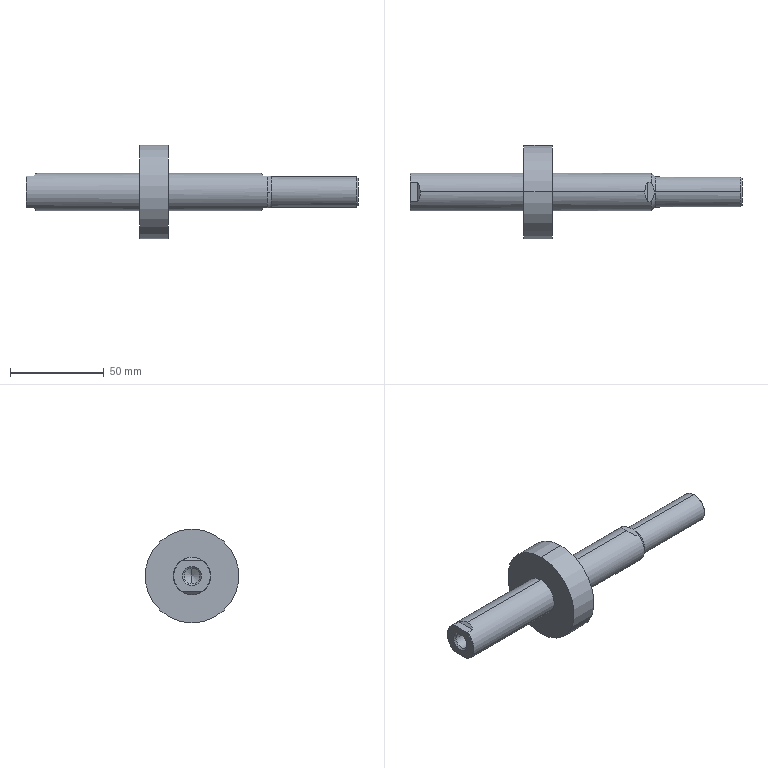Part | SolidWorks | features BaseBody 1 | 1 solid | 32 faces | box 177 x 50 x 50 mm | volume 73758 mm3 | plane 12 | cylinder 10 | cone 10 | commonest cylinder face diameters 20 x4 8.376 x2 16 x2 50 x2
STEP:
#1=CARTESIAN_POINT('',(52.75,0.,10.));
#2=VERTEX_POINT('',#1);
#3=CARTESIAN_POINT('',(52.75,0.,-10.));
#4=VERTEX_POINT('',#3);
#5=CARTESIAN_POINT('',(52.75,0.,0.));
#6=DIRECTION('',(-1.,0.,0.));
#7=DIRECTION('',(0.,0.,1.));
#8=AXIS2_PLACEMENT_3D('',#5,#6,#7);
#9=CIRCLE('',#8,10.);
#10=EDGE_CURVE('',#2,#4,#9,.T.);
#11=ORIENTED_EDGE('',*,*,#10,.T.);
#12=CARTESIAN_POINT('',(-2.5,0.,-10.));
#13=VERTEX_POINT('',#12);
#14=CARTESIAN_POINT('',(0.,0.,-10.));
#15=DIRECTION('',(-1.,0.,0.));
#16=VECTOR('',#15,1000.);
#17=LINE('',#14,#16);
#18=EDGE_CURVE('',#4,#13,#17,.T.);
#19=ORIENTED_EDGE('',*,*,#18,.T.);
#20=CARTESIAN_POINT('',(-4.,5.268,-8.5));
#21=VERTEX_POINT('',#20);
#22=CARTESIAN_POINT('',(-2.5,0.,-10.));
#23=CARTESIAN_POINT('',(-2.5,1.873,-10.));
#24=CARTESIAN_POINT('',(-3.013,3.675,-9.487));
#25=CARTESIAN_POINT('',(-4.,5.268,-8.5));
#26=(BOUNDED_CURVE()B_SPLINE_CURVE(3,(#22,#23,#24,#25),.UNSPECIFIED.,.F.,.F.)B_SPLINE_CURVE_WITH_KNOTS((4,4),(3.142,3.696),.UNSPECIFIED.)CURVE()GEOMETRIC_REPRESENTATION_ITEM()RATIONAL_B_SPLINE_CURVE((1.,0.9745,0.9745,1.))REPRESENTATION_ITEM(''));
#27=EDGE_CURVE('',#13,#21,#26,.T.);
#28=ORIENTED_EDGE('',*,*,#27,.T.);
#29=CARTESIAN_POINT('',(-7.75,5.268,-8.5));
#30=VERTEX_POINT('',#29);
#31=CARTESIAN_POINT('',(0.,5.268,-8.5));
#32=DIRECTION('',(-1.,0.,0.));
#33=VECTOR('',#32,1000.);
#34=LINE('',#31,#33);
#35=EDGE_CURVE('',#21,#30,#34,.T.);
#36=ORIENTED_EDGE('',*,*,#35,.T.);
#37=CARTESIAN_POINT('',(-7.75,5.268,8.5));
#38=VERTEX_POINT('',#37);
#39=CARTESIAN_POINT('',(-7.75,0.,0.));
#40=DIRECTION('',(1.,0.,0.));
#41=DIRECTION('',(0.,0.,1.));
#42=AXIS2_PLACEMENT_3D('',#39,#40,#41);
#43=CIRCLE('',#42,10.);
#44=EDGE_CURVE('',#30,#38,#43,.T.);
#45=ORIENTED_EDGE('',*,*,#44,.T.);
#46=CARTESIAN_POINT('',(-4.,5.268,8.5));
#47=VERTEX_POINT('',#46);
#48=CARTESIAN_POINT('',(0.,5.268,8.5));
#49=DIRECTION('',(1.,0.,0.));
#50=VECTOR('',#49,1000.);
#51=LINE('',#48,#50);
#52=EDGE_CURVE('',#38,#47,#51,.T.);
#53=ORIENTED_EDGE('',*,*,#52,.T.);
#54=CARTESIAN_POINT('',(-2.5,0.,10.));
#55=VERTEX_POINT('',#54);
#56=CARTESIAN_POINT('',(-4.,5.268,8.5));
#57=CARTESIAN_POINT('',(-3.013,3.675,9.487));
#58=CARTESIAN_POINT('',(-2.5,1.873,10.));
#59=CARTESIAN_POINT('',(-2.5,0.,10.));
#60=(BOUNDED_CURVE()B_SPLINE_CURVE(3,(#56,#57,#58,#59),.UNSPECIFIED.,.F.,.F.)B_SPLINE_CURVE_WITH_KNOTS((4,4),(2.587,3.142),.UNSPECIFIED.)CURVE()GEOMETRIC_REPRESENTATION_ITEM()RATIONAL_B_SPLINE_CURVE((1.,0.9745,0.9745,1.))REPRESENTATION_ITEM(''));
#61=EDGE_CURVE('',#47,#55,#60,.T.);
#62=ORIENTED_EDGE('',*,*,#61,.T.);
#63=CARTESIAN_POINT('',(0.,0.,10.));
#64=DIRECTION('',(-1.,0.,0.));
#65=VECTOR('',#64,1000.);
#66=LINE('',#63,#65);
#67=EDGE_CURVE('',#2,#55,#66,.T.);
#68=ORIENTED_EDGE('',*,*,#67,.F.);
#69=EDGE_LOOP('',(#11,#19,#28,#36,#45,#53,#62,#68));
#70=FACE_OUTER_BOUND('',#69,.T.);
#71=CARTESIAN_POINT('',(0.,0.,0.));
#72=DIRECTION('',(-1.,0.,0.));
#73=DIRECTION('',(0.,0.,1.));
#74=AXIS2_PLACEMENT_3D('',#71,#72,#73);
#75=CYLINDRICAL_SURFACE('',#74,10.);
#76=ADVANCED_FACE('',(#70),#75,.T.);
#77=CARTESIAN_POINT('',(67.75,0.,25.));
#78=VERTEX_POINT('',#77);
#79=CARTESIAN_POINT('',(67.75,0.,-25.));
#80=VERTEX_POINT('',#79);
#81=CARTESIAN_POINT('',(67.75,0.,0.));
#82=DIRECTION('',(-1.,0.,0.));
#83=DIRECTION('',(0.,0.,1.));
#84=AXIS2_PLACEMENT_3D('',#81,#82,#83);
#85=CIRCLE('',#84,25.);
#86=EDGE_CURVE('',#78,#80,#85,.T.);
#87=ORIENTED_EDGE('',*,*,#86,.T.);
#88=CARTESIAN_POINT('',(52.75,0.,-25.));
#89=VERTEX_POINT('',#88);
#90=CARTESIAN_POINT('',(67.75,0.,-25.));
#91=DIRECTION('',(-1.,0.,0.));
#92=VECTOR('',#91,1000.);
#93=LINE('',#90,#92);
#94=EDGE_CURVE('',#80,#89,#93,.T.);
#95=ORIENTED_EDGE('',*,*,#94,.T.);
#96=CARTESIAN_POINT('',(52.75,0.,25.));
#97=VERTEX_POINT('',#96);
#98=CARTESIAN_POINT('',(52.75,0.,0.));
#99=DIRECTION('',(1.,0.,0.));
#100=DIRECTION('',(0.,0.,1.));
#101=AXIS2_PLACEMENT_3D('',#98,#99,#100);
#102=CIRCLE('',#101,25.);
#103=EDGE_CURVE('',#89,#97,#102,.T.);
#104=ORIENTED_EDGE('',*,*,#103,.T.);
#105=CARTESIAN_POINT('',(67.75,0.,25.));
#106=DIRECTION('',(-1.,0.,0.));
#107=VECTOR('',#106,1000.);
#108=LINE('',#105,#107);
#109=EDGE_CURVE('',#78,#97,#108,.T.);
#110=ORIENTED_EDGE('',*,*,#109,.F.);
#111=EDGE_LOOP('',(#87,#95,#104,#110));
#112=FACE_OUTER_BOUND('',#111,.T.);
#113=CARTESIAN_POINT('',(67.75,0.,0.));
#114=DIRECTION('',(-1.,0.,0.));
#115=DIRECTION('',(0.,0.,1.));
#116=AXIS2_PLACEMENT_3D('',#113,#114,#115);
#117=CYLINDRICAL_SURFACE('',#116,25.);
#118=ADVANCED_FACE('',(#112),#117,.T.);
#119=CARTESIAN_POINT('',(-7.188,0.,-4.188));
#120=VERTEX_POINT('',#119);
#121=CARTESIAN_POINT('',(-7.188,-4.188,0.));
#122=VERTEX_POINT('',#121);
#123=CARTESIAN_POINT('',(-7.188,0.,0.));
#124=DIRECTION('',(-1.,0.,0.));
#125=DIRECTION('',(0.,-1.,0.));
#126=AXIS2_PLACEMENT_3D('',#123,#124,#125);
#127=CIRCLE('',#126,4.188);
#128=EDGE_CURVE('',#120,#122,#127,.T.);
#129=ORIENTED_EDGE('',*,*,#128,.F.);
#130=CARTESIAN_POINT('',(-8.,0.,-5.));
#131=VERTEX_POINT('',#130);
#132=CARTESIAN_POINT('',(-8.,0.,-5.));
#133=DIRECTION('',(-0.7071,0.,-0.7071));
#134=VECTOR('',#133,1000.);
#135=LINE('',#132,#134);
#136=EDGE_CURVE('',#120,#131,#135,.T.);
#137=ORIENTED_EDGE('',*,*,#136,.T.);
#138=CARTESIAN_POINT('',(-8.,0.,5.));
#139=VERTEX_POINT('',#138);
#140=CARTESIAN_POINT('',(-8.,0.,0.));
#141=DIRECTION('',(-1.,0.,0.));
#142=DIRECTION('',(0.,0.,1.));
#143=AXIS2_PLACEMENT_3D('',#140,#141,#142);
#144=CIRCLE('',#143,5.);
#145=EDGE_CURVE('',#131,#139,#144,.T.);
#146=ORIENTED_EDGE('',*,*,#145,.T.);
#147=CARTESIAN_POINT('',(-7.188,0.,4.188));
#148=VERTEX_POINT('',#147);
#149=CARTESIAN_POINT('',(-8.,0.,5.));
#150=DIRECTION('',(-0.7071,0.,0.7071));
#151=VECTOR('',#150,1000.);
#152=LINE('',#149,#151);
#153=EDGE_CURVE('',#148,#139,#152,.T.);
#154=ORIENTED_EDGE('',*,*,#153,.F.);
#155=CARTESIAN_POINT('',(-7.188,0.,0.));
#156=DIRECTION('',(-1.,0.,0.));
#157=DIRECTION('',(0.,-1.,0.));
#158=AXIS2_PLACEMENT_3D('',#155,#156,#157);
#159=CIRCLE('',#158,4.188);
#160=EDGE_CURVE('',#122,#148,#159,.T.);
#161=ORIENTED_EDGE('',*,*,#160,.F.);
#162=EDGE_LOOP('',(#129,#137,#146,#154,#161));
#163=FACE_OUTER_BOUND('',#162,.T.);
#164=CARTESIAN_POINT('',(-8.,0.,0.));
#165=DIRECTION('',(-1.,0.,0.));
#166=DIRECTION('',(0.,0.,1.));
#167=AXIS2_PLACEMENT_3D('',#164,#165,#166);
#168=CONICAL_SURFACE('',#167,5.,0.7854);
#169=ADVANCED_FACE('',(#163),#168,.F.);
#170=CARTESIAN_POINT('',(10.,4.188,0.));
#171=VERTEX_POINT('',#170);
#172=CARTESIAN_POINT('',(10.,0.,-4.188));
#173=VERTEX_POINT('',#172);
#174=CARTESIAN_POINT('',(10.,0.,0.));
#175=DIRECTION('',(-1.,0.,0.));
#176=DIRECTION('',(0.,-1.,0.));
#177=AXIS2_PLACEMENT_3D('',#174,#175,#176);
#178=CIRCLE('',#177,4.188);
#179=EDGE_CURVE('',#171,#173,#178,.T.);
#180=ORIENTED_EDGE('',*,*,#179,.F.);
#181=CARTESIAN_POINT('',(-7.188,4.188,0.));
#182=VERTEX_POINT('',#181);
#183=CARTESIAN_POINT('',(12.418,4.188,0.));
#184=DIRECTION('',(-1.,0.,0.));
#185=VECTOR('',#184,1000.);
#186=LINE('',#183,#185);
#187=EDGE_CURVE('',#171,#182,#186,.T.);
#188=ORIENTED_EDGE('',*,*,#187,.T.);
#189=CARTESIAN_POINT('',(-7.188,0.,0.));
#190=DIRECTION('',(-1.,0.,0.));
#191=DIRECTION('',(0.,-1.,0.));
#192=AXIS2_PLACEMENT_3D('',#189,#190,#191);
#193=CIRCLE('',#192,4.188);
#194=EDGE_CURVE('',#182,#120,#193,.T.);
#195=ORIENTED_EDGE('',*,*,#194,.T.);
#196=ORIENTED_EDGE('',*,*,#128,.T.);
#197=CARTESIAN_POINT('',(10.,-4.188,0.));
#198=VERTEX_POINT('',#197);
#199=CARTESIAN_POINT('',(12.418,-4.188,0.));
#200=DIRECTION('',(-1.,0.,0.));
#201=VECTOR('',#200,1000.);
#202=LINE('',#199,#201);
#203=EDGE_CURVE('',#198,#122,#202,.T.);
#204=ORIENTED_EDGE('',*,*,#203,.F.);
#205=CARTESIAN_POINT('',(10.,0.,0.));
#206=DIRECTION('',(-1.,0.,0.));
#207=DIRECTION('',(0.,-1.,0.));
#208=AXIS2_PLACEMENT_3D('',#205,#206,#207);
#209=CIRCLE('',#208,4.188);
#210=EDGE_CURVE('',#173,#198,#209,.T.);
#211=ORIENTED_EDGE('',*,*,#210,.F.);
#212=EDGE_LOOP('',(#180,#188,#195,#196,#204,#211));
#213=FACE_OUTER_BOUND('',#212,.T.);
#214=CARTESIAN_POINT('',(12.418,0.,0.));
#215=DIRECTION('',(-1.,0.,0.));
#216=DIRECTION('',(0.,-1.,0.));
#217=AXIS2_PLACEMENT_3D('',#214,#215,#216);
#218=CYLINDRICAL_SURFACE('',#217,4.188);
#219=ADVANCED_FACE('',(#213),#218,.F.);
#220=CARTESIAN_POINT('',(118.7,5.268,-8.5));
#221=VERTEX_POINT('',#220);
#222=CARTESIAN_POINT('',(117.2,0.,-10.));
#223=VERTEX_POINT('',#222);
#224=CARTESIAN_POINT('',(118.7,5.268,-8.5));
#225=CARTESIAN_POINT('',(117.713,3.675,-9.487));
#226=CARTESIAN_POINT('',(117.2,1.873,-10.));
#227=CARTESIAN_POINT('',(117.2,0.,-10.));
#228=(BOUNDED_CURVE()B_SPLINE_CURVE(3,(#224,#225,#226,#227),.UNSPECIFIED.,.F.,.F.)B_SPLINE_CURVE_WITH_KNOTS((4,4),(5.728,6.283),.UNSPECIFIED.)CURVE()GEOMETRIC_REPRESENTATION_ITEM()RATIONAL_B_SPLINE_CURVE((1.,0.9745,0.9745,1.))REPRESENTATION_ITEM(''));
#229=EDGE_CURVE('',#221,#223,#228,.T.);
#230=ORIENTED_EDGE('',*,*,#229,.T.);
#231=CARTESIAN_POINT('',(67.75,0.,-10.));
#232=VERTEX_POINT('',#231);
#233=CARTESIAN_POINT('',(169.,0.,-10.));
#234=DIRECTION('',(-1.,0.,0.));
#235=VECTOR('',#234,1000.);
#236=LINE('',#233,#235);
#237=EDGE_CURVE('',#223,#232,#236,.T.);
#238=ORIENTED_EDGE('',*,*,#237,.T.);
#239=CARTESIAN_POINT('',(67.75,0.,10.));
#240=VERTEX_POINT('',#239);
#241=CARTESIAN_POINT('',(67.75,0.,0.));
#242=DIRECTION('',(1.,0.,0.));
#243=DIRECTION('',(0.,0.,1.));
#244=AXIS2_PLACEMENT_3D('',#241,#242,#243);
#245=CIRCLE('',#244,10.);
#246=EDGE_CURVE('',#232,#240,#245,.T.);
#247=ORIENTED_EDGE('',*,*,#246,.T.);
#248=CARTESIAN_POINT('',(117.2,0.,10.));
#249=VERTEX_POINT('',#248);
#250=CARTESIAN_POINT('',(169.,0.,10.));
#251=DIRECTION('',(-1.,0.,0.));
#252=VECTOR('',#251,1000.);
#253=LINE('',#250,#252);
#254=EDGE_CURVE('',#249,#240,#253,.T.);
#255=ORIENTED_EDGE('',*,*,#254,.F.);
#256=CARTESIAN_POINT('',(118.7,5.268,8.5));
#257=VERTEX_POINT('',#256);
#258=CARTESIAN_POINT('',(117.2,0.,10.));
#259=CARTESIAN_POINT('',(117.2,1.873,10.));
#260=CARTESIAN_POINT('',(117.713,3.675,9.487));
#261=CARTESIAN_POINT('',(118.7,5.268,8.5));
#262=(BOUNDED_CURVE()B_SPLINE_CURVE(3,(#258,#259,#260,#261),.UNSPECIFIED.,.F.,.F.)B_SPLINE_CURVE_WITH_KNOTS((4,4),(0.,0.5548),.UNSPECIFIED.)CURVE()GEOMETRIC_REPRESENTATION_ITEM()RATIONAL_B_SPLINE_CURVE((1.,0.9745,0.9745,1.))REPRESENTATION_ITEM(''));
#263=EDGE_CURVE('',#249,#257,#262,.T.);
#264=ORIENTED_EDGE('',*,*,#263,.T.);
#265=CARTESIAN_POINT('',(120.7,5.268,8.5));
#266=VERTEX_POINT('',#265);
#267=CARTESIAN_POINT('',(169.,5.268,8.5));
#268=DIRECTION('',(1.,0.,0.));
#269=VECTOR('',#268,1000.);
#270=LINE('',#267,#269);
#271=EDGE_CURVE('',#257,#266,#270,.T.);
#272=ORIENTED_EDGE('',*,*,#271,.T.);
#273=CARTESIAN_POINT('',(120.7,10.,0.));
#274=VERTEX_POINT('',#273);
#275=CARTESIAN_POINT('',(120.7,0.,0.));
#276=DIRECTION('',(-1.,0.,0.));
#277=DIRECTION('',(0.,0.,1.));
#278=AXIS2_PLACEMENT_3D('',#275,#276,#277);
#279=CIRCLE('',#278,10.);
#280=EDGE_CURVE('',#266,#274,#279,.T.);
#281=ORIENTED_EDGE('',*,*,#280,.T.);
#282=CARTESIAN_POINT('',(120.7,5.268,-8.5));
#283=VERTEX_POINT('',#282);
#284=CARTESIAN_POINT('',(120.7,0.,0.));
#285=DIRECTION('',(-1.,0.,0.));
#286=DIRECTION('',(0.,0.,1.));
#287=AXIS2_PLACEMENT_3D('',#284,#285,#286);
#288=CIRCLE('',#287,10.);
#289=EDGE_CURVE('',#274,#283,#288,.T.);
#290=ORIENTED_EDGE('',*,*,#289,.T.);
#291=CARTESIAN_POINT('',(169.,5.268,-8.5));
#292=DIRECTION('',(-1.,0.,0.));
#293=VECTOR('',#292,1000.);
#294=LINE('',#291,#293);
#295=EDGE_CURVE('',#283,#221,#294,.T.);
#296=ORIENTED_EDGE('',*,*,#295,.T.);
#297=EDGE_LOOP('',(#230,#238,#247,#255,#264,#272,#281,#290,#296));
#298=FACE_OUTER_BOUND('',#297,.T.);
#299=CARTESIAN_POINT('',(169.,0.,0.));
#300=DIRECTION('',(-1.,0.,0.));
#301=DIRECTION('',(0.,0.,1.));
#302=AXIS2_PLACEMENT_3D('',#299,#300,#301);
#303=CYLINDRICAL_SURFACE('',#302,10.);
#304=ADVANCED_FACE('',(#298),#303,.T.);
#305=CARTESIAN_POINT('',(12.418,0.,0.));
#306=VERTEX_POINT('',#305);
#307=CARTESIAN_POINT('',(10.,0.,4.188));
#308=VERTEX_POINT('',#307);
#309=CARTESIAN_POINT('',(10.,0.,4.188));
#310=DIRECTION('',(-0.5,0.,0.866));
#311=VECTOR('',#310,1000.);
#312=LINE('',#309,#311);
#313=EDGE_CURVE('',#306,#308,#312,.T.);
#314=ORIENTED_EDGE('',*,*,#313,.F.);
#315=CARTESIAN_POINT('',(10.,0.,-4.188));
#316=DIRECTION('',(-0.5,0.,-0.866));
#317=VECTOR('',#316,1000.);
#318=LINE('',#315,#317);
#319=EDGE_CURVE('',#306,#173,#318,.T.);
#320=ORIENTED_EDGE('',*,*,#319,.T.);
#321=ORIENTED_EDGE('',*,*,#210,.T.);
#322=CARTESIAN_POINT('',(10.,0.,0.));
#323=DIRECTION('',(-1.,0.,0.));
#324=DIRECTION('',(0.,-1.,0.));
#325=AXIS2_PLACEMENT_3D('',#322,#323,#324);
#326=CIRCLE('',#325,4.188);
#327=EDGE_CURVE('',#198,#308,#326,.T.);
#328=ORIENTED_EDGE('',*,*,#327,.T.);
#329=EDGE_LOOP('',(#314,#320,#321,#328));
#330=FACE_OUTER_BOUND('',#329,.T.);
#331=CARTESIAN_POINT('',(10.,0.,0.));
#332=DIRECTION('',(-1.,0.,0.));
#333=DIRECTION('',(0.,0.,1.));
#334=AXIS2_PLACEMENT_3D('',#331,#332,#333);
#335=CONICAL_SURFACE('',#334,4.188,1.047);
#336=ADVANCED_FACE('',(#330),#335,.F.);
#337=CARTESIAN_POINT('',(122.7,0.,8.));
#338=VERTEX_POINT('',#337);
#339=CARTESIAN_POINT('',(122.7,8.,0.));
#340=VERTEX_POINT('',#339);
#341=CARTESIAN_POINT('',(122.7,0.,0.));
#342=DIRECTION('',(-1.,0.,0.));
#343=DIRECTION('',(0.,0.,1.));
#344=AXIS2_PLACEMENT_3D('',#341,#342,#343);
#345=CIRCLE('',#344,8.);
#346=EDGE_CURVE('',#338,#340,#345,.T.);
#347=ORIENTED_EDGE('',*,*,#346,.T.);
#348=CARTESIAN_POINT('',(120.7,10.,0.));
#349=DIRECTION('',(-0.7071,0.7071,0.));
#350=VECTOR('',#349,1000.);
#351=LINE('',#348,#350);
#352=EDGE_CURVE('',#340,#274,#351,.T.);
#353=ORIENTED_EDGE('',*,*,#352,.T.);
#354=ORIENTED_EDGE('',*,*,#280,.F.);
#355=CARTESIAN_POINT('',(120.7,-5.268,8.5));
#356=VERTEX_POINT('',#355);
#357=CARTESIAN_POINT('',(120.7,-5.268,8.5));
#358=CARTESIAN_POINT('',(121.132,-4.448,8.5));
#359=CARTESIAN_POINT('',(121.504,-3.607,8.5));
#360=CARTESIAN_POINT('',(121.907,-2.289,8.5));
#361=CARTESIAN_POINT('',(122.015,-1.838,8.5));
#362=CARTESIAN_POINT('',(122.162,-0.919,8.5));
#363=CARTESIAN_POINT('',(122.2,-0.4598,8.5));
#364=CARTESIAN_POINT('',(122.2,0.4584,8.5));
#365=CARTESIAN_POINT('',(122.163,0.9173,8.5));
#366=CARTESIAN_POINT('',(122.016,1.835,8.5));
#367=CARTESIAN_POINT('',(121.908,2.287,8.5));
#368=CARTESIAN_POINT('',(121.505,3.606,8.5));
#369=CARTESIAN_POINT('',(121.132,4.448,8.5));
#370=CARTESIAN_POINT('',(120.7,5.268,8.5));
#371=B_SPLINE_CURVE_WITH_KNOTS('',3,(#357,#358,#359,#360,#361,#362,#363,#364,#365,#366,#367,#368,#369,#370),.UNSPECIFIED.,.F.,.F.,(4,2,2,2,2,2,4),(0.,0.002753,0.00413,0.005507,0.006884,0.00826,0.01101),.UNSPECIFIED.);
#372=EDGE_CURVE('',#356,#266,#371,.T.);
#373=ORIENTED_EDGE('',*,*,#372,.F.);
#374=CARTESIAN_POINT('',(120.7,-10.,0.));
#375=VERTEX_POINT('',#374);
#376=CARTESIAN_POINT('',(120.7,0.,0.));
#377=DIRECTION('',(-1.,0.,0.));
#378=DIRECTION('',(0.,0.,1.));
#379=AXIS2_PLACEMENT_3D('',#376,#377,#378);
#380=CIRCLE('',#379,10.);
#381=EDGE_CURVE('',#375,#356,#380,.T.);
#382=ORIENTED_EDGE('',*,*,#381,.F.);
#383=CARTESIAN_POINT('',(122.7,-8.,0.));
#384=VERTEX_POINT('',#383);
#385=CARTESIAN_POINT('',(120.7,-10.,0.));
#386=DIRECTION('',(-0.7071,-0.7071,0.));
#387=VECTOR('',#386,1000.);
#388=LINE('',#385,#387);
#389=EDGE_CURVE('',#384,#375,#388,.T.);
#390=ORIENTED_EDGE('',*,*,#389,.F.);
#391=CARTESIAN_POINT('',(122.7,0.,0.));
#392=DIRECTION('',(-1.,0.,0.));
#393=DIRECTION('',(0.,0.,1.));
#394=AXIS2_PLACEMENT_3D('',#391,#392,#393);
#395=CIRCLE('',#394,8.);
#396=EDGE_CURVE('',#384,#338,#395,.T.);
#397=ORIENTED_EDGE('',*,*,#396,.T.);
#398=EDGE_LOOP('',(#347,#353,#354,#373,#382,#390,#397));
#399=FACE_OUTER_BOUND('',#398,.T.);
#400=CARTESIAN_POINT('',(120.7,0.,0.));
#401=DIRECTION('',(-1.,0.,0.));
#402=DIRECTION('',(0.,-1.,0.));
#403=AXIS2_PLACEMENT_3D('',#400,#401,#402);
#404=CONICAL_SURFACE('',#403,10.,0.7854);
#405=ADVANCED_FACE('',(#399),#404,.T.);
#406=CARTESIAN_POINT('',(168.08,0.,8.));
#407=VERTEX_POINT('',#406);
#408=CARTESIAN_POINT('',(168.08,0.,-8.));
#409=VERTEX_POINT('',#408);
#410=CARTESIAN_POINT('',(168.08,0.,0.));
#411=DIRECTION('',(-1.,0.,0.));
#412=DIRECTION('',(0.,0.,1.));
#413=AXIS2_PLACEMENT_3D('',#410,#411,#412);
#414=CIRCLE('',#413,8.);
#415=EDGE_CURVE('',#407,#409,#414,.T.);
#416=ORIENTED_EDGE('',*,*,#415,.T.);
#417=CARTESIAN_POINT('',(122.7,0.,-8.));
#418=VERTEX_POINT('',#417);
#419=CARTESIAN_POINT('',(169.,0.,-8.));
#420=DIRECTION('',(-1.,0.,0.));
#421=VECTOR('',#420,1000.);
#422=LINE('',#419,#421);
#423=EDGE_CURVE('',#409,#418,#422,.T.);
#424=ORIENTED_EDGE('',*,*,#423,.T.);
#425=CARTESIAN_POINT('',(122.7,0.,0.));
#426=DIRECTION('',(-1.,0.,0.));
#427=DIRECTION('',(0.,0.,1.));
#428=AXIS2_PLACEMENT_3D('',#425,#426,#427);
#429=CIRCLE('',#428,8.);
#430=EDGE_CURVE('',#340,#418,#429,.T.);
#431=ORIENTED_EDGE('',*,*,#430,.F.);
#432=ORIENTED_EDGE('',*,*,#346,.F.);
#433=CARTESIAN_POINT('',(169.,0.,8.));
#434=DIRECTION('',(-1.,0.,0.));
#435=VECTOR('',#434,1000.);
#436=LINE('',#433,#435);
#437=EDGE_CURVE('',#407,#338,#436,.T.);
#438=ORIENTED_EDGE('',*,*,#437,.F.);
#439=EDGE_LOOP('',(#416,#424,#431,#432,#438));
#440=FACE_OUTER_BOUND('',#439,.T.);
#441=CARTESIAN_POINT('',(169.,0.,0.));
#442=DIRECTION('',(-1.,0.,0.));
#443=DIRECTION('',(0.,0.,1.));
#444=AXIS2_PLACEMENT_3D('',#441,#442,#443);
#445=CYLINDRICAL_SURFACE('',#444,8.);
#446=ADVANCED_FACE('',(#440),#445,.T.);
#447=CARTESIAN_POINT('',(169.,0.,7.08));
#448=VERTEX_POINT('',#447);
#449=CARTESIAN_POINT('',(169.,0.,-7.08));
#450=VERTEX_POINT('',#449);
#451=CARTESIAN_POINT('',(169.,0.,0.));
#452=DIRECTION('',(-1.,0.,0.));
#453=DIRECTION('',(0.,0.,1.));
#454=AXIS2_PLACEMENT_3D('',#451,#452,#453);
#455=CIRCLE('',#454,7.08);
#456=EDGE_CURVE('',#448,#450,#455,.T.);
#457=ORIENTED_EDGE('',*,*,#456,.T.);
#458=CARTESIAN_POINT('',(168.08,0.,-8.));
#459=DIRECTION('',(-0.7071,0.,-0.7071));
#460=VECTOR('',#459,1000.);
#461=LINE('',#458,#460);
#462=EDGE_CURVE('',#450,#409,#461,.T.);
#463=ORIENTED_EDGE('',*,*,#462,.T.);
#464=ORIENTED_EDGE('',*,*,#415,.F.);
#465=CARTESIAN_POINT('',(168.08,0.,8.));
#466=DIRECTION('',(-0.7071,0.,0.7071));
#467=VECTOR('',#466,1000.);
#468=LINE('',#465,#467);
#469=EDGE_CURVE('',#448,#407,#468,.T.);
#470=ORIENTED_EDGE('',*,*,#469,.F.);
#471=EDGE_LOOP('',(#457,#463,#464,#470));
#472=FACE_OUTER_BOUND('',#471,.T.);
#473=CARTESIAN_POINT('',(168.08,0.,0.));
#474=DIRECTION('',(-1.,0.,0.));
#475=DIRECTION('',(0.,0.,1.));
#476=AXIS2_PLACEMENT_3D('',#473,#474,#475);
#477=CONICAL_SURFACE('',#476,8.,0.7854);
#478=ADVANCED_FACE('',(#472),#477,.T.);
#479=ORIENTED_EDGE('',*,*,#18,.F.);
#480=CARTESIAN_POINT('',(52.75,0.,0.));
#481=DIRECTION('',(-1.,0.,0.));
#482=DIRECTION('',(0.,0.,1.));
#483=AXIS2_PLACEMENT_3D('',#480,#481,#482);
#484=CIRCLE('',#483,10.);
#485=EDGE_CURVE('',#4,#2,#484,.T.);
#486=ORIENTED_EDGE('',*,*,#485,.T.);
#487=ORIENTED_EDGE('',*,*,#67,.T.);
#488=CARTESIAN_POINT('',(-4.,-5.268,8.5));
#489=VERTEX_POINT('',#488);
#490=CARTESIAN_POINT('',(-2.5,0.,10.));
#491=CARTESIAN_POINT('',(-2.5,-1.873,10.));
#492=CARTESIAN_POINT('',(-3.013,-3.675,9.487));
#493=CARTESIAN_POINT('',(-4.,-5.268,8.5));
#494=(BOUNDED_CURVE()B_SPLINE_CURVE(3,(#490,#491,#492,#493),.UNSPECIFIED.,.F.,.F.)B_SPLINE_CURVE_WITH_KNOTS((4,4),(3.142,3.696),.UNSPECIFIED.)CURVE()GEOMETRIC_REPRESENTATION_ITEM()RATIONAL_B_SPLINE_CURVE((1.,0.9745,0.9745,1.))REPRESENTATION_ITEM(''));
#495=EDGE_CURVE('',#55,#489,#494,.T.);
#496=ORIENTED_EDGE('',*,*,#495,.T.);
#497=CARTESIAN_POINT('',(-7.75,-5.268,8.5));
#498=VERTEX_POINT('',#497);
#499=CARTESIAN_POINT('',(0.,-5.268,8.5));
#500=DIRECTION('',(-1.,0.,0.));
#501=VECTOR('',#500,1000.);
#502=LINE('',#499,#501);
#503=EDGE_CURVE('',#489,#498,#502,.T.);
#504=ORIENTED_EDGE('',*,*,#503,.T.);
#505=CARTESIAN_POINT('',(-7.75,-5.268,-8.5));
#506=VERTEX_POINT('',#505);
#507=CARTESIAN_POINT('',(-7.75,0.,0.));
#508=DIRECTION('',(1.,0.,0.));
#509=DIRECTION('',(0.,0.,1.));
#510=AXIS2_PLACEMENT_3D('',#507,#508,#509);
#511=CIRCLE('',#510,10.);
#512=EDGE_CURVE('',#498,#506,#511,.T.);
#513=ORIENTED_EDGE('',*,*,#512,.T.);
#514=CARTESIAN_POINT('',(-4.,-5.268,-8.5));
#515=VERTEX_POINT('',#514);
#516=CARTESIAN_POINT('',(0.,-5.268,-8.5));
#517=DIRECTION('',(1.,0.,0.));
#518=VECTOR('',#517,1000.);
#519=LINE('',#516,#518);
#520=EDGE_CURVE('',#506,#515,#519,.T.);
#521=ORIENTED_EDGE('',*,*,#520,.T.);
#522=CARTESIAN_POINT('',(-4.,-5.268,-8.5));
#523=CARTESIAN_POINT('',(-3.013,-3.675,-9.487));
#524=CARTESIAN_POINT('',(-2.5,-1.873,-10.));
#525=CARTESIAN_POINT('',(-2.5,0.,-10.));
#526=(BOUNDED_CURVE()B_SPLINE_CURVE(3,(#522,#523,#524,#525),.UNSPECIFIED.,.F.,.F.)B_SPLINE_CURVE_WITH_KNOTS((4,4),(2.587,3.142),.UNSPECIFIED.)CURVE()GEOMETRIC_REPRESENTATION_ITEM()RATIONAL_B_SPLINE_CURVE((1.,0.9745,0.9745,1.))REPRESENTATION_ITEM(''));
#527=EDGE_CURVE('',#515,#13,#526,.T.);
#528=ORIENTED_EDGE('',*,*,#527,.T.);
#529=EDGE_LOOP('',(#479,#486,#487,#496,#504,#513,#521,#528));
#530=FACE_OUTER_BOUND('',#529,.T.);
#531=CARTESIAN_POINT('',(0.,0.,0.));
#532=DIRECTION('',(-1.,0.,0.));
#533=DIRECTION('',(0.,0.,1.));
#534=AXIS2_PLACEMENT_3D('',#531,#532,#533);
#535=CYLINDRICAL_SURFACE('',#534,10.);
#536=ADVANCED_FACE('',(#530),#535,.T.);
#537=ORIENTED_EDGE('',*,*,#527,.F.);
#538=CARTESIAN_POINT('',(-4.,17.,-8.5));
#539=DIRECTION('',(0.,1.,0.));
#540=VECTOR('',#539,1000.);
#541=LINE('',#538,#540);
#542=EDGE_CURVE('',#515,#21,#541,.T.);
#543=ORIENTED_EDGE('',*,*,#542,.T.);
#544=ORIENTED_EDGE('',*,*,#27,.F.);
#545=EDGE_LOOP('',(#537,#543,#544));
#546=FACE_OUTER_BOUND('',#545,.T.);
#547=CARTESIAN_POINT('',(-4.,17.,-8.5));
#548=DIRECTION('',(-0.7071,0.,-0.7071));
#549=DIRECTION('',(-0.7071,0.,0.7071));
#550=AXIS2_PLACEMENT_3D('',#547,#548,#549);
#551=PLANE('',#550);
#552=ADVANCED_FACE('',(#546),#551,.T.);
#553=CARTESIAN_POINT('',(-8.,-4.776,-8.5));
#554=VERTEX_POINT('',#553);
#555=CARTESIAN_POINT('',(-7.75,-5.268,-8.5));
#556=CARTESIAN_POINT('',(-7.837,-5.102,-8.5));
#557=CARTESIAN_POINT('',(-7.921,-4.938,-8.5));
#558=CARTESIAN_POINT('',(-8.,-4.776,-8.5));
#559=B_SPLINE_CURVE_WITH_KNOTS('',3,(#555,#556,#557,#558),.UNSPECIFIED.,.F.,.F.,(4,4),(0.,1.),.UNSPECIFIED.);
#560=EDGE_CURVE('',#506,#554,#559,.T.);
#561=ORIENTED_EDGE('',*,*,#560,.T.);
#562=CARTESIAN_POINT('',(-8.,4.776,-8.5));
#563=VERTEX_POINT('',#562);
#564=CARTESIAN_POINT('',(-8.,17.,-8.5));
#565=DIRECTION('',(0.,1.,0.));
#566=VECTOR('',#565,1000.);
#567=LINE('',#564,#566);
#568=EDGE_CURVE('',#554,#563,#567,.T.);
#569=ORIENTED_EDGE('',*,*,#568,.T.);
#570=CARTESIAN_POINT('',(-8.,4.776,-8.5));
#571=CARTESIAN_POINT('',(-7.921,4.938,-8.5));
#572=CARTESIAN_POINT('',(-7.837,5.102,-8.5));
#573=CARTESIAN_POINT('',(-7.75,5.268,-8.5));
#574=B_SPLINE_CURVE_WITH_KNOTS('',3,(#570,#571,#572,#573),.UNSPECIFIED.,.F.,.F.,(4,4),(0.,1.),.UNSPECIFIED.);
#575=EDGE_CURVE('',#563,#30,#574,.T.);
#576=ORIENTED_EDGE('',*,*,#575,.T.);
#577=ORIENTED_EDGE('',*,*,#35,.F.);
#578=ORIENTED_EDGE('',*,*,#542,.F.);
#579=ORIENTED_EDGE('',*,*,#520,.F.);
#580=EDGE_LOOP('',(#561,#569,#576,#577,#578,#579));
#581=FACE_OUTER_BOUND('',#580,.T.);
#582=CARTESIAN_POINT('',(-8.,17.,-8.5));
#583=DIRECTION('',(0.,0.,-1.));
#584=DIRECTION('',(-1.,0.,0.));
#585=AXIS2_PLACEMENT_3D('',#582,#583,#584);
#586=PLANE('',#585);
#587=ADVANCED_FACE('',(#581),#586,.T.);
#588=ORIENTED_EDGE('',*,*,#560,.F.);
#589=ORIENTED_EDGE('',*,*,#512,.F.);
#590=CARTESIAN_POINT('',(-8.,-4.776,8.5));
#591=VERTEX_POINT('',#590);
#592=CARTESIAN_POINT('',(-7.75,-5.268,8.5));
#593=CARTESIAN_POINT('',(-7.837,-5.103,8.5));
#594=CARTESIAN_POINT('',(-7.92,-4.939,8.5));
#595=CARTESIAN_POINT('',(-8.,-4.776,8.5));
#596=B_SPLINE_CURVE_WITH_KNOTS('',3,(#592,#593,#594,#595),.UNSPECIFIED.,.F.,.F.,(4,4),(0.,1.),.UNSPECIFIED.);
#597=EDGE_CURVE('',#498,#591,#596,.T.);
#598=ORIENTED_EDGE('',*,*,#597,.T.);
#599=CARTESIAN_POINT('',(-8.,0.,0.));
#600=DIRECTION('',(1.,0.,0.));
#601=DIRECTION('',(0.,0.,-1.));
#602=AXIS2_PLACEMENT_3D('',#599,#600,#601);
#603=CIRCLE('',#602,9.75);
#604=EDGE_CURVE('',#591,#554,#603,.T.);
#605=ORIENTED_EDGE('',*,*,#604,.T.);
#606=EDGE_LOOP('',(#588,#589,#598,#605));
#607=FACE_OUTER_BOUND('',#606,.T.);
#608=CARTESIAN_POINT('',(-7.75,0.,0.));
#609=DIRECTION('',(1.,0.,0.));
#610=DIRECTION('',(0.,0.,-1.));
#611=AXIS2_PLACEMENT_3D('',#608,#609,#610);
#612=CONICAL_SURFACE('',#611,10.,0.7854);
#613=ADVANCED_FACE('',(#607),#612,.T.);
#614=CARTESIAN_POINT('',(-8.,4.776,8.5));
#615=VERTEX_POINT('',#614);
#616=CARTESIAN_POINT('',(-7.75,5.268,8.5));
#617=CARTESIAN_POINT('',(-7.837,5.102,8.5));
#618=CARTESIAN_POINT('',(-7.921,4.938,8.5));
#619=CARTESIAN_POINT('',(-8.,4.776,8.5));
#620=B_SPLINE_CURVE_WITH_KNOTS('',3,(#616,#617,#618,#619),.UNSPECIFIED.,.F.,.F.,(4,4),(0.,1.),.UNSPECIFIED.);
#621=EDGE_CURVE('',#38,#615,#620,.T.);
#622=ORIENTED_EDGE('',*,*,#621,.T.);
#623=CARTESIAN_POINT('',(-8.,17.,8.5));
#624=DIRECTION('',(0.,-1.,0.));
#625=VECTOR('',#624,1000.);
#626=LINE('',#623,#625);
#627=EDGE_CURVE('',#615,#591,#626,.T.);
#628=ORIENTED_EDGE('',*,*,#627,.T.);
#629=ORIENTED_EDGE('',*,*,#597,.F.);
#630=ORIENTED_EDGE('',*,*,#503,.F.);
#631=CARTESIAN_POINT('',(-4.,17.,8.5));
#632=DIRECTION('',(0.,1.,0.));
#633=VECTOR('',#632,1000.);
#634=LINE('',#631,#633);
#635=EDGE_CURVE('',#489,#47,#634,.T.);
#636=ORIENTED_EDGE('',*,*,#635,.T.);
#637=ORIENTED_EDGE('',*,*,#52,.F.);
#638=EDGE_LOOP('',(#622,#628,#629,#630,#636,#637));
#639=FACE_OUTER_BOUND('',#638,.T.);
#640=CARTESIAN_POINT('',(-4.,17.,8.5));
#641=DIRECTION('',(0.,0.,1.));
#642=DIRECTION('',(1.,0.,0.));
#643=AXIS2_PLACEMENT_3D('',#640,#641,#642);
#644=PLANE('',#643);
#645=ADVANCED_FACE('',(#639),#644,.T.);
#646=ORIENTED_EDGE('',*,*,#61,.F.);
#647=ORIENTED_EDGE('',*,*,#635,.F.);
#648=ORIENTED_EDGE('',*,*,#495,.F.);
#649=EDGE_LOOP('',(#646,#647,#648));
#650=FACE_OUTER_BOUND('',#649,.T.);
#651=CARTESIAN_POINT('',(1.,17.,13.5));
#652=DIRECTION('',(-0.7071,0.,0.7071));
#653=DIRECTION('',(0.7071,0.,0.7071));
#654=AXIS2_PLACEMENT_3D('',#651,#652,#653);
#655=PLANE('',#654);
#656=ADVANCED_FACE('',(#650),#655,.T.);
#657=ORIENTED_EDGE('',*,*,#621,.F.);
#658=ORIENTED_EDGE('',*,*,#44,.F.);
#659=ORIENTED_EDGE('',*,*,#575,.F.);
#660=CARTESIAN_POINT('',(-8.,0.,0.));
#661=DIRECTION('',(1.,0.,0.));
#662=DIRECTION('',(0.,0.,-1.));
#663=AXIS2_PLACEMENT_3D('',#660,#661,#662);
#664=CIRCLE('',#663,9.75);
#665=EDGE_CURVE('',#563,#615,#664,.T.);
#666=ORIENTED_EDGE('',*,*,#665,.T.);
#667=EDGE_LOOP('',(#657,#658,#659,#666));
#668=FACE_OUTER_BOUND('',#667,.T.);
#669=CARTESIAN_POINT('',(-7.75,0.,0.));
#670=DIRECTION('',(1.,0.,0.));
#671=DIRECTION('',(0.,0.,-1.));
#672=AXIS2_PLACEMENT_3D('',#669,#670,#671);
#673=CONICAL_SURFACE('',#672,10.,0.7854);
#674=ADVANCED_FACE('',(#668),#673,.T.);
#675=ORIENTED_EDGE('',*,*,#10,.F.);
#676=ORIENTED_EDGE('',*,*,#485,.F.);
#677=EDGE_LOOP('',(#675,#676));
#678=FACE_BOUND('',#677,.T.);
#679=CARTESIAN_POINT('',(52.75,0.,0.));
#680=DIRECTION('',(1.,0.,0.));
#681=DIRECTION('',(0.,0.,1.));
#682=AXIS2_PLACEMENT_3D('',#679,#680,#681);
#683=CIRCLE('',#682,25.);
#684=EDGE_CURVE('',#97,#89,#683,.T.);
#685=ORIENTED_EDGE('',*,*,#684,.F.);
#686=ORIENTED_EDGE('',*,*,#103,.F.);
#687=EDGE_LOOP('',(#685,#686));
#688=FACE_OUTER_BOUND('',#687,.T.);
#689=CARTESIAN_POINT('',(52.75,10.,0.));
#690=DIRECTION('',(1.,0.,0.));
#691=DIRECTION('',(0.,0.,-1.));
#692=AXIS2_PLACEMENT_3D('',#689,#690,#691);
#693=PLANE('',#692);
#694=ADVANCED_FACE('',(#678,#688),#693,.F.);
#695=CARTESIAN_POINT('',(-8.,0.,0.));
#696=DIRECTION('',(-1.,0.,0.));
#697=DIRECTION('',(0.,0.,1.));
#698=AXIS2_PLACEMENT_3D('',#695,#696,#697);
#699=CIRCLE('',#698,5.);
#700=EDGE_CURVE('',#139,#131,#699,.T.);
#701=ORIENTED_EDGE('',*,*,#700,.F.);
#702=ORIENTED_EDGE('',*,*,#145,.F.);
#703=EDGE_LOOP('',(#701,#702));
#704=FACE_BOUND('',#703,.T.);
#705=ORIENTED_EDGE('',*,*,#568,.F.);
#706=ORIENTED_EDGE('',*,*,#604,.F.);
#707=ORIENTED_EDGE('',*,*,#627,.F.);
#708=ORIENTED_EDGE('',*,*,#665,.F.);
#709=EDGE_LOOP('',(#705,#706,#707,#708));
#710=FACE_OUTER_BOUND('',#709,.T.);
#711=CARTESIAN_POINT('',(-8.,0.,0.));
#712=DIRECTION('',(1.,0.,0.));
#713=DIRECTION('',(0.,0.,-1.));
#714=AXIS2_PLACEMENT_3D('',#711,#712,#713);
#715=PLANE('',#714);
#716=ADVANCED_FACE('',(#704,#710),#715,.F.);
#717=ORIENTED_EDGE('',*,*,#94,.F.);
#718=CARTESIAN_POINT('',(67.75,0.,0.));
#719=DIRECTION('',(-1.,0.,0.));
#720=DIRECTION('',(0.,0.,1.));
#721=AXIS2_PLACEMENT_3D('',#718,#719,#720);
#722=CIRCLE('',#721,25.);
#723=EDGE_CURVE('',#80,#78,#722,.T.);
#724=ORIENTED_EDGE('',*,*,#723,.T.);
#725=ORIENTED_EDGE('',*,*,#109,.T.);
#726=ORIENTED_EDGE('',*,*,#684,.T.);
#727=EDGE_LOOP('',(#717,#724,#725,#726));
#728=FACE_OUTER_BOUND('',#727,.T.);
#729=CARTESIAN_POINT('',(67.75,0.,0.));
#730=DIRECTION('',(-1.,0.,0.));
#731=DIRECTION('',(0.,0.,1.));
#732=AXIS2_PLACEMENT_3D('',#729,#730,#731);
#733=CYLINDRICAL_SURFACE('',#732,25.);
#734=ADVANCED_FACE('',(#728),#733,.T.);
#735=ORIENTED_EDGE('',*,*,#136,.F.);
#736=ORIENTED_EDGE('',*,*,#194,.F.);
#737=CARTESIAN_POINT('',(-7.188,0.,0.));
#738=DIRECTION('',(-1.,0.,0.));
#739=DIRECTION('',(0.,-1.,0.));
#740=AXIS2_PLACEMENT_3D('',#737,#738,#739);
#741=CIRCLE('',#740,4.188);
#742=EDGE_CURVE('',#148,#182,#741,.T.);
#743=ORIENTED_EDGE('',*,*,#742,.F.);
#744=ORIENTED_EDGE('',*,*,#153,.T.);
#745=ORIENTED_EDGE('',*,*,#700,.T.);
#746=EDGE_LOOP('',(#735,#736,#743,#744,#745));
#747=FACE_OUTER_BOUND('',#746,.T.);
#748=CARTESIAN_POINT('',(-8.,0.,0.));
#749=DIRECTION('',(-1.,0.,0.));
#750=DIRECTION('',(0.,0.,1.));
#751=AXIS2_PLACEMENT_3D('',#748,#749,#750);
#752=CONICAL_SURFACE('',#751,5.,0.7854);
#753=ADVANCED_FACE('',(#747),#752,.F.);
#754=ORIENTED_EDGE('',*,*,#86,.F.);
#755=ORIENTED_EDGE('',*,*,#723,.F.);
#756=EDGE_LOOP('',(#754,#755));
#757=FACE_OUTER_BOUND('',#756,.T.);
#758=CARTESIAN_POINT('',(67.75,0.,0.));
#759=DIRECTION('',(1.,0.,0.));
#760=DIRECTION('',(0.,0.,1.));
#761=AXIS2_PLACEMENT_3D('',#758,#759,#760);
#762=CIRCLE('',#761,10.);
#763=EDGE_CURVE('',#240,#232,#762,.T.);
#764=ORIENTED_EDGE('',*,*,#763,.F.);
#765=ORIENTED_EDGE('',*,*,#246,.F.);
#766=EDGE_LOOP('',(#764,#765));
#767=FACE_BOUND('',#766,.T.);
#768=CARTESIAN_POINT('',(67.75,25.,0.));
#769=DIRECTION('',(-1.,0.,0.));
#770=DIRECTION('',(0.,0.,1.));
#771=AXIS2_PLACEMENT_3D('',#768,#769,#770);
#772=PLANE('',#771);
#773=ADVANCED_FACE('',(#757,#767),#772,.F.);
#774=ORIENTED_EDGE('',*,*,#187,.F.);
#775=CARTESIAN_POINT('',(10.,0.,0.));
#776=DIRECTION('',(-1.,0.,0.));
#777=DIRECTION('',(0.,-1.,0.));
#778=AXIS2_PLACEMENT_3D('',#775,#776,#777);
#779=CIRCLE('',#778,4.188);
#780=EDGE_CURVE('',#308,#171,#779,.T.);
#781=ORIENTED_EDGE('',*,*,#780,.F.);
#782=ORIENTED_EDGE('',*,*,#327,.F.);
#783=ORIENTED_EDGE('',*,*,#203,.T.);
#784=ORIENTED_EDGE('',*,*,#160,.T.);
#785=ORIENTED_EDGE('',*,*,#742,.T.);
#786=EDGE_LOOP('',(#774,#781,#782,#783,#784,#785));
#787=FACE_OUTER_BOUND('',#786,.T.);
#788=CARTESIAN_POINT('',(12.418,0.,0.));
#789=DIRECTION('',(-1.,0.,0.));
#790=DIRECTION('',(0.,-1.,0.));
#791=AXIS2_PLACEMENT_3D('',#788,#789,#790);
#792=CYLINDRICAL_SURFACE('',#791,4.188);
#793=ADVANCED_FACE('',(#787),#792,.F.);
#794=ORIENTED_EDGE('',*,*,#237,.F.);
#795=CARTESIAN_POINT('',(118.7,-5.268,-8.5));
#796=VERTEX_POINT('',#795);
#797=CARTESIAN_POINT('',(117.2,0.,-10.));
#798=CARTESIAN_POINT('',(117.2,-1.873,-10.));
#799=CARTESIAN_POINT('',(117.713,-3.675,-9.487));
#800=CARTESIAN_POINT('',(118.7,-5.268,-8.5));
#801=(BOUNDED_CURVE()B_SPLINE_CURVE(3,(#797,#798,#799,#800),.UNSPECIFIED.,.F.,.F.)B_SPLINE_CURVE_WITH_KNOTS((4,4),(0.,0.5548),.UNSPECIFIED.)CURVE()GEOMETRIC_REPRESENTATION_ITEM()RATIONAL_B_SPLINE_CURVE((1.,0.9745,0.9745,1.))REPRESENTATION_ITEM(''));
#802=EDGE_CURVE('',#223,#796,#801,.T.);
#803=ORIENTED_EDGE('',*,*,#802,.T.);
#804=CARTESIAN_POINT('',(120.7,-5.268,-8.5));
#805=VERTEX_POINT('',#804);
#806=CARTESIAN_POINT('',(169.,-5.268,-8.5));
#807=DIRECTION('',(1.,0.,0.));
#808=VECTOR('',#807,1000.);
#809=LINE('',#806,#808);
#810=EDGE_CURVE('',#796,#805,#809,.T.);
#811=ORIENTED_EDGE('',*,*,#810,.T.);
#812=CARTESIAN_POINT('',(120.7,0.,0.));
#813=DIRECTION('',(-1.,0.,0.));
#814=DIRECTION('',(0.,0.,1.));
#815=AXIS2_PLACEMENT_3D('',#812,#813,#814);
#816=CIRCLE('',#815,10.);
#817=EDGE_CURVE('',#805,#375,#816,.T.);
#818=ORIENTED_EDGE('',*,*,#817,.T.);
#819=ORIENTED_EDGE('',*,*,#381,.T.);
#820=CARTESIAN_POINT('',(118.7,-5.268,8.5));
#821=VERTEX_POINT('',#820);
#822=CARTESIAN_POINT('',(169.,-5.268,8.5));
#823=DIRECTION('',(-1.,0.,0.));
#824=VECTOR('',#823,1000.);
#825=LINE('',#822,#824);
#826=EDGE_CURVE('',#356,#821,#825,.T.);
#827=ORIENTED_EDGE('',*,*,#826,.T.);
#828=CARTESIAN_POINT('',(118.7,-5.268,8.5));
#829=CARTESIAN_POINT('',(117.713,-3.675,9.487));
#830=CARTESIAN_POINT('',(117.2,-1.873,10.));
#831=CARTESIAN_POINT('',(117.2,0.,10.));
#832=(BOUNDED_CURVE()B_SPLINE_CURVE(3,(#828,#829,#830,#831),.UNSPECIFIED.,.F.,.F.)B_SPLINE_CURVE_WITH_KNOTS((4,4),(5.728,6.283),.UNSPECIFIED.)CURVE()GEOMETRIC_REPRESENTATION_ITEM()RATIONAL_B_SPLINE_CURVE((1.,0.9745,0.9745,1.))REPRESENTATION_ITEM(''));
#833=EDGE_CURVE('',#821,#249,#832,.T.);
#834=ORIENTED_EDGE('',*,*,#833,.T.);
#835=ORIENTED_EDGE('',*,*,#254,.T.);
#836=ORIENTED_EDGE('',*,*,#763,.T.);
#837=EDGE_LOOP('',(#794,#803,#811,#818,#819,#827,#834,#835,#836));
#838=FACE_OUTER_BOUND('',#837,.T.);
#839=CARTESIAN_POINT('',(169.,0.,0.));
#840=DIRECTION('',(-1.,0.,0.));
#841=DIRECTION('',(0.,0.,1.));
#842=AXIS2_PLACEMENT_3D('',#839,#840,#841);
#843=CYLINDRICAL_SURFACE('',#842,10.);
#844=ADVANCED_FACE('',(#838),#843,.T.);
#845=ORIENTED_EDGE('',*,*,#319,.F.);
#846=ORIENTED_EDGE('',*,*,#313,.T.);
#847=ORIENTED_EDGE('',*,*,#780,.T.);
#848=ORIENTED_EDGE('',*,*,#179,.T.);
#849=EDGE_LOOP('',(#845,#846,#847,#848));
#850=FACE_OUTER_BOUND('',#849,.T.);
#851=CARTESIAN_POINT('',(10.,0.,0.));
#852=DIRECTION('',(-1.,0.,0.));
#853=DIRECTION('',(0.,0.,1.));
#854=AXIS2_PLACEMENT_3D('',#851,#852,#853);
#855=CONICAL_SURFACE('',#854,4.188,1.047);
#856=ADVANCED_FACE('',(#850),#855,.F.);
#857=ORIENTED_EDGE('',*,*,#271,.F.);
#858=CARTESIAN_POINT('',(118.7,17.,8.5));
#859=DIRECTION('',(0.,-1.,0.));
#860=VECTOR('',#859,1000.);
#861=LINE('',#858,#860);
#862=EDGE_CURVE('',#257,#821,#861,.T.);
#863=ORIENTED_EDGE('',*,*,#862,.T.);
#864=ORIENTED_EDGE('',*,*,#826,.F.);
#865=ORIENTED_EDGE('',*,*,#372,.T.);
#866=EDGE_LOOP('',(#857,#863,#864,#865));
#867=FACE_OUTER_BOUND('',#866,.T.);
#868=CARTESIAN_POINT('',(122.7,17.,8.5));
#869=DIRECTION('',(0.,0.,1.));
#870=DIRECTION('',(1.,0.,0.));
#871=AXIS2_PLACEMENT_3D('',#868,#869,#870);
#872=PLANE('',#871);
#873=ADVANCED_FACE('',(#867),#872,.T.);
#874=ORIENTED_EDGE('',*,*,#833,.F.);
#875=ORIENTED_EDGE('',*,*,#862,.F.);
#876=ORIENTED_EDGE('',*,*,#263,.F.);
#877=EDGE_LOOP('',(#874,#875,#876));
#878=FACE_OUTER_BOUND('',#877,.T.);
#879=CARTESIAN_POINT('',(118.7,17.,8.5));
#880=DIRECTION('',(0.7071,0.,0.7071));
#881=DIRECTION('',(0.7071,0.,-0.7071));
#882=AXIS2_PLACEMENT_3D('',#879,#880,#881);
#883=PLANE('',#882);
#884=ADVANCED_FACE('',(#878),#883,.T.);
#885=ORIENTED_EDGE('',*,*,#352,.F.);
#886=ORIENTED_EDGE('',*,*,#430,.T.);
#887=CARTESIAN_POINT('',(122.7,0.,0.));
#888=DIRECTION('',(-1.,0.,0.));
#889=DIRECTION('',(0.,0.,1.));
#890=AXIS2_PLACEMENT_3D('',#887,#888,#889);
#891=CIRCLE('',#890,8.);
#892=EDGE_CURVE('',#418,#384,#891,.T.);
#893=ORIENTED_EDGE('',*,*,#892,.T.);
#894=ORIENTED_EDGE('',*,*,#389,.T.);
#895=ORIENTED_EDGE('',*,*,#817,.F.);
#896=CARTESIAN_POINT('',(120.7,-5.268,-8.5));
#897=CARTESIAN_POINT('',(121.132,-4.448,-8.5));
#898=CARTESIAN_POINT('',(121.504,-3.607,-8.5));
#899=CARTESIAN_POINT('',(121.907,-2.289,-8.5));
#900=CARTESIAN_POINT('',(122.015,-1.838,-8.5));
#901=CARTESIAN_POINT('',(122.162,-0.919,-8.5));
#902=CARTESIAN_POINT('',(122.2,-0.4598,-8.5));
#903=CARTESIAN_POINT('',(122.2,0.4584,-8.5));
#904=CARTESIAN_POINT('',(122.163,0.9173,-8.5));
#905=CARTESIAN_POINT('',(122.016,1.835,-8.5));
#906=CARTESIAN_POINT('',(121.908,2.287,-8.5));
#907=CARTESIAN_POINT('',(121.505,3.606,-8.5));
#908=CARTESIAN_POINT('',(121.132,4.448,-8.5));
#909=CARTESIAN_POINT('',(120.7,5.268,-8.5));
#910=B_SPLINE_CURVE_WITH_KNOTS('',3,(#896,#897,#898,#899,#900,#901,#902,#903,#904,#905,#906,#907,#908,#909),.UNSPECIFIED.,.F.,.F.,(4,2,2,2,2,2,4),(0.,0.002753,0.00413,0.005507,0.006884,0.00826,0.01101),.UNSPECIFIED.);
#911=EDGE_CURVE('',#805,#283,#910,.T.);
#912=ORIENTED_EDGE('',*,*,#911,.T.);
#913=ORIENTED_EDGE('',*,*,#289,.F.);
#914=EDGE_LOOP('',(#885,#886,#893,#894,#895,#912,#913));
#915=FACE_OUTER_BOUND('',#914,.T.);
#916=CARTESIAN_POINT('',(120.7,0.,0.));
#917=DIRECTION('',(-1.,0.,0.));
#918=DIRECTION('',(0.,-1.,0.));
#919=AXIS2_PLACEMENT_3D('',#916,#917,#918);
#920=CONICAL_SURFACE('',#919,10.,0.7854);
#921=ADVANCED_FACE('',(#915),#920,.T.);
#922=ORIENTED_EDGE('',*,*,#810,.F.);
#923=CARTESIAN_POINT('',(118.7,17.,-8.5));
#924=DIRECTION('',(0.,1.,0.));
#925=VECTOR('',#924,1000.);
#926=LINE('',#923,#925);
#927=EDGE_CURVE('',#796,#221,#926,.T.);
#928=ORIENTED_EDGE('',*,*,#927,.T.);
#929=ORIENTED_EDGE('',*,*,#295,.F.);
#930=ORIENTED_EDGE('',*,*,#911,.F.);
#931=EDGE_LOOP('',(#922,#928,#929,#930));
#932=FACE_OUTER_BOUND('',#931,.T.);
#933=CARTESIAN_POINT('',(118.7,17.,-8.5));
#934=DIRECTION('',(0.,0.,-1.));
#935=DIRECTION('',(-1.,0.,0.));
#936=AXIS2_PLACEMENT_3D('',#933,#934,#935);
#937=PLANE('',#936);
#938=ADVANCED_FACE('',(#932),#937,.T.);
#939=ORIENTED_EDGE('',*,*,#229,.F.);
#940=ORIENTED_EDGE('',*,*,#927,.F.);
#941=ORIENTED_EDGE('',*,*,#802,.F.);
#942=EDGE_LOOP('',(#939,#940,#941));
#943=FACE_OUTER_BOUND('',#942,.T.);
#944=CARTESIAN_POINT('',(111.629,17.,-15.571));
#945=DIRECTION('',(0.7071,0.,-0.7071));
#946=DIRECTION('',(-0.7071,0.,-0.7071));
#947=AXIS2_PLACEMENT_3D('',#944,#945,#946);
#948=PLANE('',#947);
#949=ADVANCED_FACE('',(#943),#948,.T.);
#950=ORIENTED_EDGE('',*,*,#423,.F.);
#951=CARTESIAN_POINT('',(168.08,0.,0.));
#952=DIRECTION('',(-1.,0.,0.));
#953=DIRECTION('',(0.,0.,1.));
#954=AXIS2_PLACEMENT_3D('',#951,#952,#953);
#955=CIRCLE('',#954,8.);
#956=EDGE_CURVE('',#409,#407,#955,.T.);
#957=ORIENTED_EDGE('',*,*,#956,.T.);
#958=ORIENTED_EDGE('',*,*,#437,.T.);
#959=ORIENTED_EDGE('',*,*,#396,.F.);
#960=ORIENTED_EDGE('',*,*,#892,.F.);
#961=EDGE_LOOP('',(#950,#957,#958,#959,#960));
#962=FACE_OUTER_BOUND('',#961,.T.);
#963=CARTESIAN_POINT('',(169.,0.,0.));
#964=DIRECTION('',(-1.,0.,0.));
#965=DIRECTION('',(0.,0.,1.));
#966=AXIS2_PLACEMENT_3D('',#963,#964,#965);
#967=CYLINDRICAL_SURFACE('',#966,8.);
#968=ADVANCED_FACE('',(#962),#967,.T.);
#969=ORIENTED_EDGE('',*,*,#462,.F.);
#970=CARTESIAN_POINT('',(169.,0.,0.));
#971=DIRECTION('',(-1.,0.,0.));
#972=DIRECTION('',(0.,0.,1.));
#973=AXIS2_PLACEMENT_3D('',#970,#971,#972);
#974=CIRCLE('',#973,7.08);
#975=EDGE_CURVE('',#450,#448,#974,.T.);
#976=ORIENTED_EDGE('',*,*,#975,.T.);
#977=ORIENTED_EDGE('',*,*,#469,.T.);
#978=ORIENTED_EDGE('',*,*,#956,.F.);
#979=EDGE_LOOP('',(#969,#976,#977,#978));
#980=FACE_OUTER_BOUND('',#979,.T.);
#981=CARTESIAN_POINT('',(168.08,0.,0.));
#982=DIRECTION('',(-1.,0.,0.));
#983=DIRECTION('',(0.,0.,1.));
#984=AXIS2_PLACEMENT_3D('',#981,#982,#983);
#985=CONICAL_SURFACE('',#984,8.,0.7854);
#986=ADVANCED_FACE('',(#980),#985,.T.);
#987=ORIENTED_EDGE('',*,*,#456,.F.);
#988=ORIENTED_EDGE('',*,*,#975,.F.);
#989=EDGE_LOOP('',(#987,#988));
#990=FACE_OUTER_BOUND('',#989,.T.);
#991=CARTESIAN_POINT('',(169.,7.08,0.));
#992=DIRECTION('',(-1.,0.,0.));
#993=DIRECTION('',(0.,0.,1.));
#994=AXIS2_PLACEMENT_3D('',#991,#992,#993);
#995=PLANE('',#994);
#996=ADVANCED_FACE('',(#990),#995,.F.);
#997=CLOSED_SHELL('',(#76,#118,#169,#219,#304,#336,#405,#446,#478,#536,#552,#587,#613,#645,#656,#674,#694,#716,#734,#753,#773,#793,#844,#856,#873,#884,#921,#938,#949,#968,#986,#996));
#998=MANIFOLD_SOLID_BREP('',#997);
#999=CARTESIAN_POINT('',(0.,0.,0.));
#1000=DIRECTION('',(0.,0.,1.));
#1001=DIRECTION('',(1.,0.,0.));
#1002=AXIS2_PLACEMENT_3D('',#999,#1000,#1001);
#1003=(LENGTH_UNIT()NAMED_UNIT(*)SI_UNIT(.MILLI.,.METRE.));
#1004=UNCERTAINTY_MEASURE_WITH_UNIT(LENGTH_MEASURE(0.00001),#1003,'','');
#1005=(NAMED_UNIT(*)PLANE_ANGLE_UNIT()SI_UNIT($,.RADIAN.));
#1006=(NAMED_UNIT(*)SI_UNIT($,.STERADIAN.)SOLID_ANGLE_UNIT());
#1007=(GEOMETRIC_REPRESENTATION_CONTEXT(3)GLOBAL_UNCERTAINTY_ASSIGNED_CONTEXT((#1004))GLOBAL_UNIT_ASSIGNED_CONTEXT((#1003,#1005,#1006))REPRESENTATION_CONTEXT('',''));
#1008=ADVANCED_BREP_SHAPE_REPRESENTATION('',(#998,#1002),#1007);